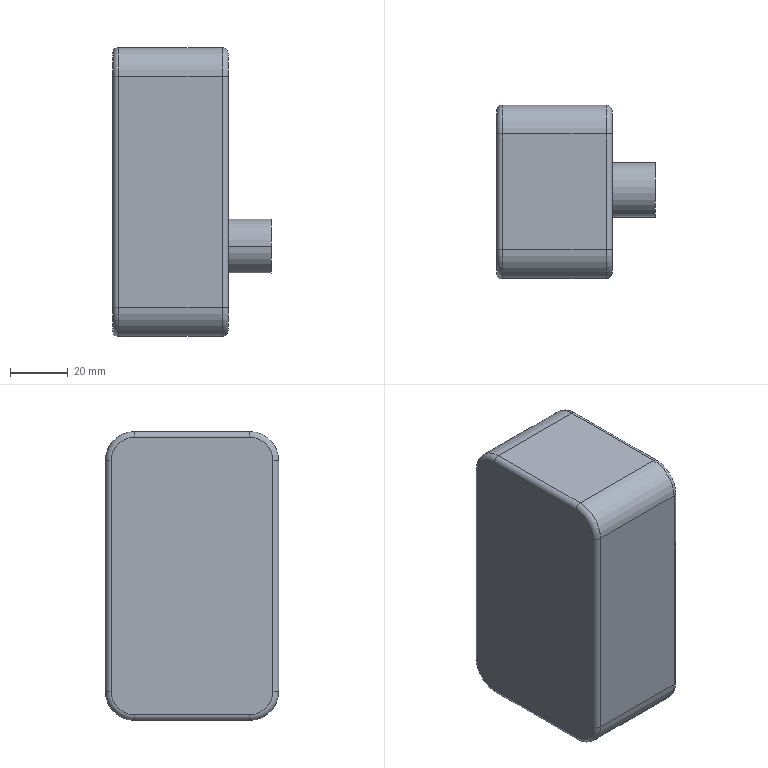Part | STEP file | PN_0014 | 1 solid | 29 faces | box 55 x 60 x 100 mm | volume 240255 mm3 | cylinder 14 | torus 8 | plane 7 | commonest cylinder face diameters 4 x8 20 x4 18.89 x2